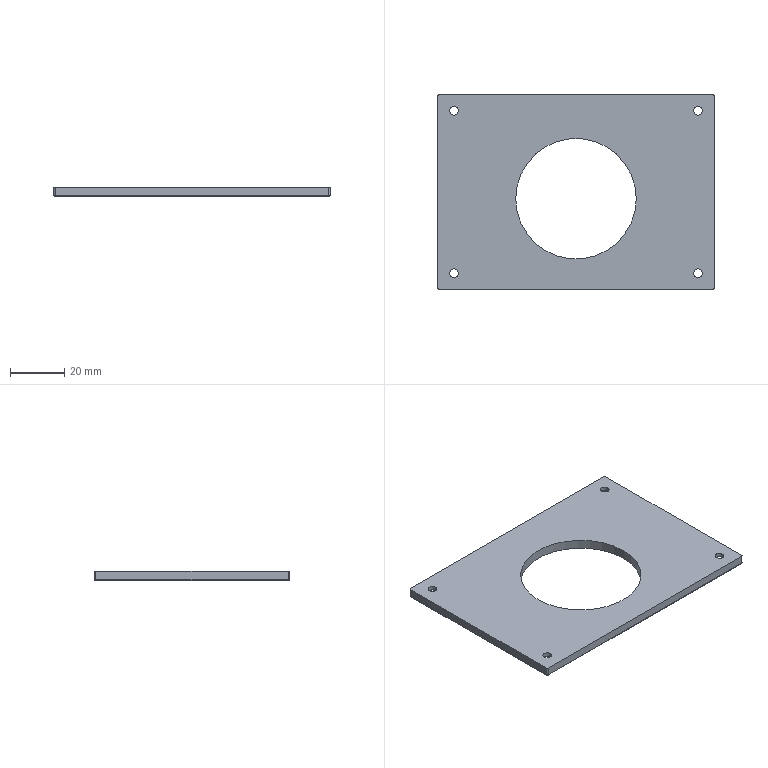Part | STEP file | Insert/withdraw label (with lock) | 1 solid | 552 faces | box 102 x 72 x 3.5 mm | volume 19316 mm3 | plane 382 | spline 134 | cylinder 32 | sphere 4 | commonest cylinder face diameters 1 x8 3.2 x8 8.5 x8 55 x3 65 x3 44.5 x2